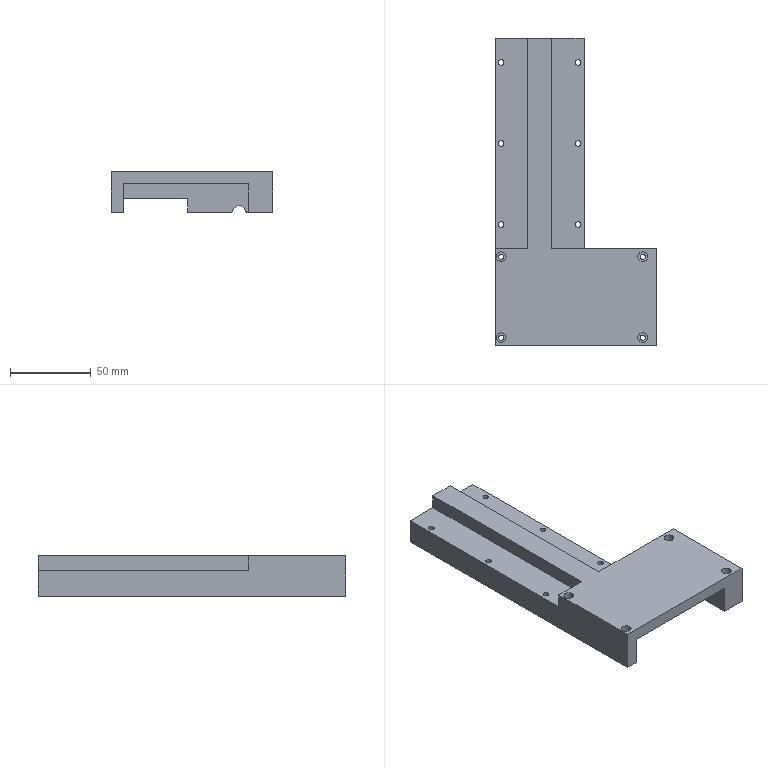Part | SolidWorks | features ICE 11, Extrusion 1, Fillet 1, MoveFace 1 | 1 solid | 57 faces | box 100 x 190 x 25 mm | volume 163793 mm3 | cylinder 32 | plane 25 | commonest cylinder face diameters 3.5 x12 3.2 x8 6.1 x8 2 x2 8 x2